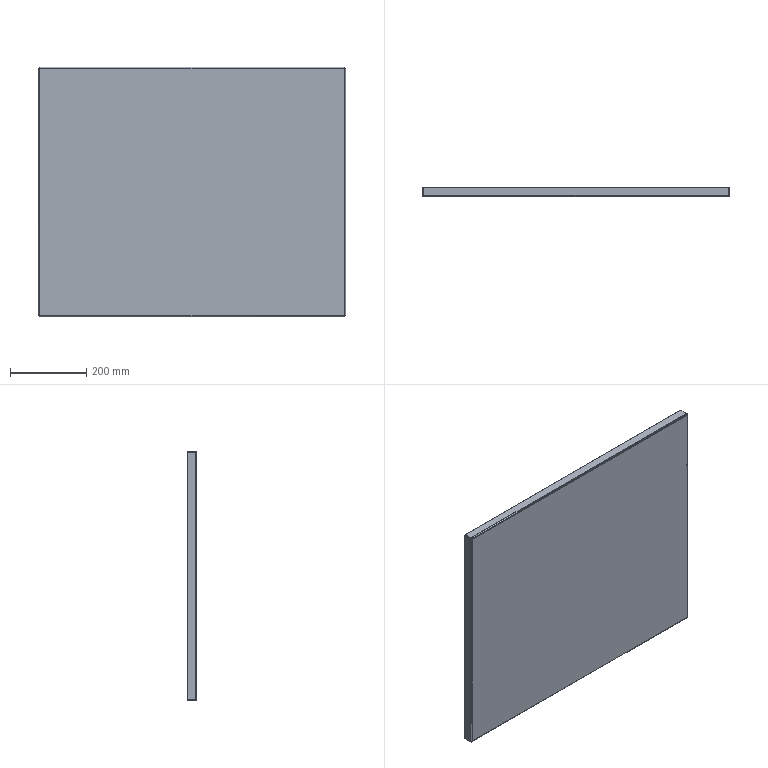Part | STEP file | Door SGN-1-10 | 1 solid | 38 faces | box 804 x 25 x 654 mm | volume 1178482 mm3 | plane 22 | spline 8 | cylinder 8 | commonest cylinder face diameters 3 x4 7 x4